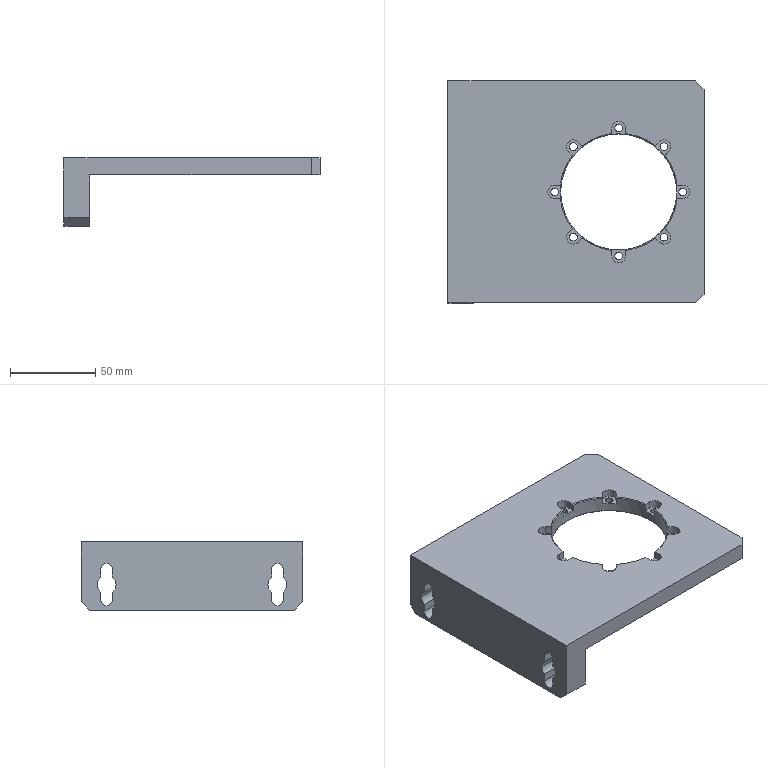Part | 1 solid | 93 faces | box 150 x 130 x 40 mm | volume 208366 mm3 | plane 44 | cylinder 39 | cone 10 | commonest cylinder face diameters 4.5 x16 8 x11 11 x6 6.6 x4 68 x2